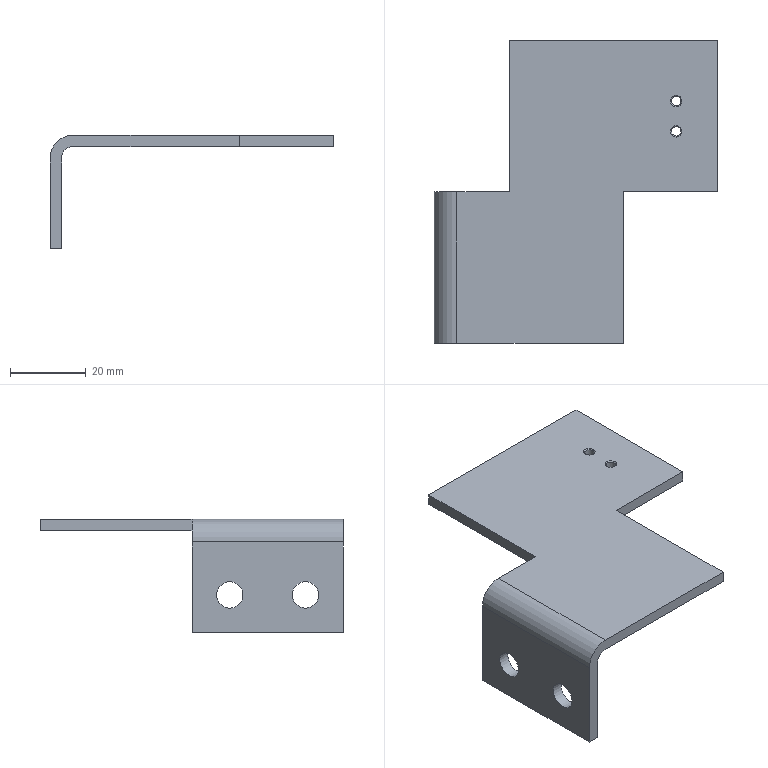Part | NX | features 5003_220_Bracket 2 | 1 solid | 20 faces | box 75 x 80 x 30 mm | volume 15347 mm3 | plane 12 | cylinder 6 | cone 2 | commonest cylinder face diameters 2.5 x2 7 x2 6 x1 12 x1
STEP:
#1=CARTESIAN_POINT('',(268.825,-58.6,-25.));
#2=VERTEX_POINT('',#1);
#3=CARTESIAN_POINT('',(268.825,-58.6,-22.));
#4=VERTEX_POINT('',#3);
#5=CARTESIAN_POINT('',(268.825,-58.6,-72.));
#6=DIRECTION('',(0.,0.,1.));
#7=VECTOR('',#6,1000.);
#8=LINE('',#5,#7);
#9=EDGE_CURVE('',#2,#4,#8,.T.);
#10=ORIENTED_EDGE('',*,*,#9,.F.);
#11=CARTESIAN_POINT('',(268.825,-18.6,-25.));
#12=VERTEX_POINT('',#11);
#13=CARTESIAN_POINT('',(268.825,-98.6,-25.));
#14=DIRECTION('',(0.,1.,0.));
#15=VECTOR('',#14,1000.);
#16=LINE('',#13,#15);
#17=EDGE_CURVE('',#2,#12,#16,.T.);
#18=ORIENTED_EDGE('',*,*,#17,.T.);
#19=CARTESIAN_POINT('',(268.825,-18.6,-22.));
#20=VERTEX_POINT('',#19);
#21=CARTESIAN_POINT('',(268.825,-18.6,-22.));
#22=DIRECTION('',(0.,0.,1.));
#23=VECTOR('',#22,1000.);
#24=LINE('',#21,#23);
#25=EDGE_CURVE('',#12,#20,#24,.T.);
#26=ORIENTED_EDGE('',*,*,#25,.T.);
#27=CARTESIAN_POINT('',(268.825,-98.6,-22.));
#28=DIRECTION('',(0.,1.,0.));
#29=VECTOR('',#28,1000.);
#30=LINE('',#27,#29);
#31=EDGE_CURVE('',#4,#20,#30,.T.);
#32=ORIENTED_EDGE('',*,*,#31,.F.);
#33=EDGE_LOOP('',(#10,#18,#26,#32));
#34=FACE_BOUND('',#33,.T.);
#35=CARTESIAN_POINT('',(268.825,-98.6,-22.));
#36=DIRECTION('',(-1.,0.,0.));
#37=DIRECTION('',(0.,-1.,0.));
#38=AXIS2_PLACEMENT_3D('',#35,#36,#37);
#39=PLANE('',#38);
#40=ADVANCED_FACE('',(#34),#39,.F.);
#41=CARTESIAN_POINT('',(257.825,-44.125,-22.));
#42=VERTEX_POINT('',#41);
#43=CARTESIAN_POINT('',(257.825,-42.6,-22.));
#44=DIRECTION('',(0.,0.,1.));
#45=DIRECTION('',(0.,-1.,0.));
#46=AXIS2_PLACEMENT_3D('',#43,#44,#45);
#47=CIRCLE('',#46,1.525);
#48=EDGE_CURVE('',#42,#42,#47,.T.);
#49=ORIENTED_EDGE('',*,*,#48,.F.);
#50=EDGE_LOOP('',(#49));
#51=FACE_BOUND('',#50,.T.);
#52=CARTESIAN_POINT('',(257.825,-36.125,-22.));
#53=VERTEX_POINT('',#52);
#54=CARTESIAN_POINT('',(257.825,-34.6,-22.));
#55=DIRECTION('',(0.,0.,1.));
#56=DIRECTION('',(0.,-1.,0.));
#57=AXIS2_PLACEMENT_3D('',#54,#55,#56);
#58=CIRCLE('',#57,1.525);
#59=EDGE_CURVE('',#53,#53,#58,.T.);
#60=ORIENTED_EDGE('',*,*,#59,.F.);
#61=EDGE_LOOP('',(#60));
#62=FACE_BOUND('',#61,.T.);
#63=CARTESIAN_POINT('',(243.825,-58.6,-22.));
#64=VERTEX_POINT('',#63);
#65=CARTESIAN_POINT('',(193.825,-58.6,-22.));
#66=DIRECTION('',(1.,0.,0.));
#67=VECTOR('',#66,1000.);
#68=LINE('',#65,#67);
#69=EDGE_CURVE('',#64,#4,#68,.T.);
#70=ORIENTED_EDGE('',*,*,#69,.T.);
#71=ORIENTED_EDGE('',*,*,#31,.T.);
#72=CARTESIAN_POINT('',(213.825,-18.6,-22.));
#73=VERTEX_POINT('',#72);
#74=CARTESIAN_POINT('',(199.825,-18.6,-22.));
#75=DIRECTION('',(-1.,0.,0.));
#76=VECTOR('',#75,1000.);
#77=LINE('',#74,#76);
#78=EDGE_CURVE('',#20,#73,#77,.T.);
#79=ORIENTED_EDGE('',*,*,#78,.T.);
#80=CARTESIAN_POINT('',(213.825,-58.6,-22.));
#81=VERTEX_POINT('',#80);
#82=CARTESIAN_POINT('',(213.825,-18.6,-22.));
#83=DIRECTION('',(0.,-1.,0.));
#84=VECTOR('',#83,1000.);
#85=LINE('',#82,#84);
#86=EDGE_CURVE('',#73,#81,#85,.T.);
#87=ORIENTED_EDGE('',*,*,#86,.T.);
#88=CARTESIAN_POINT('',(199.825,-58.6,-22.));
#89=VERTEX_POINT('',#88);
#90=CARTESIAN_POINT('',(173.825,-58.6,-22.));
#91=DIRECTION('',(1.,0.,0.));
#92=VECTOR('',#91,1000.);
#93=LINE('',#90,#92);
#94=EDGE_CURVE('',#89,#81,#93,.T.);
#95=ORIENTED_EDGE('',*,*,#94,.F.);
#96=CARTESIAN_POINT('',(199.825,-98.6,-22.));
#97=VERTEX_POINT('',#96);
#98=CARTESIAN_POINT('',(199.825,-98.6,-22.));
#99=DIRECTION('',(0.,1.,0.));
#100=VECTOR('',#99,1000.);
#101=LINE('',#98,#100);
#102=EDGE_CURVE('',#97,#89,#101,.T.);
#103=ORIENTED_EDGE('',*,*,#102,.F.);
#104=CARTESIAN_POINT('',(243.825,-98.6,-22.));
#105=VERTEX_POINT('',#104);
#106=CARTESIAN_POINT('',(199.825,-98.6,-22.));
#107=DIRECTION('',(-1.,0.,0.));
#108=VECTOR('',#107,1000.);
#109=LINE('',#106,#108);
#110=EDGE_CURVE('',#105,#97,#109,.T.);
#111=ORIENTED_EDGE('',*,*,#110,.F.);
#112=CARTESIAN_POINT('',(243.825,-18.6,-22.));
#113=DIRECTION('',(0.,-1.,0.));
#114=VECTOR('',#113,1000.);
#115=LINE('',#112,#114);
#116=EDGE_CURVE('',#64,#105,#115,.T.);
#117=ORIENTED_EDGE('',*,*,#116,.F.);
#118=EDGE_LOOP('',(#70,#71,#79,#87,#95,#103,#111,#117));
#119=FACE_BOUND('',#118,.T.);
#120=CARTESIAN_POINT('',(199.825,-98.6,-22.));
#121=DIRECTION('',(0.,0.,-1.));
#122=DIRECTION('',(0.,1.,0.));
#123=AXIS2_PLACEMENT_3D('',#120,#121,#122);
#124=PLANE('',#123);
#125=ADVANCED_FACE('',(#51,#62,#119),#124,.F.);
#126=CARTESIAN_POINT('',(257.825,-43.85,-25.));
#127=VERTEX_POINT('',#126);
#128=CARTESIAN_POINT('',(257.825,-42.6,-25.));
#129=DIRECTION('',(0.,0.,1.));
#130=DIRECTION('',(0.,-1.,0.));
#131=AXIS2_PLACEMENT_3D('',#128,#129,#130);
#132=CIRCLE('',#131,1.25);
#133=EDGE_CURVE('',#127,#127,#132,.T.);
#134=ORIENTED_EDGE('',*,*,#133,.T.);
#135=EDGE_LOOP('',(#134));
#136=FACE_BOUND('',#135,.T.);
#137=CARTESIAN_POINT('',(257.825,-35.85,-25.));
#138=VERTEX_POINT('',#137);
#139=CARTESIAN_POINT('',(257.825,-34.6,-25.));
#140=DIRECTION('',(0.,0.,1.));
#141=DIRECTION('',(0.,-1.,0.));
#142=AXIS2_PLACEMENT_3D('',#139,#140,#141);
#143=CIRCLE('',#142,1.25);
#144=EDGE_CURVE('',#138,#138,#143,.T.);
#145=ORIENTED_EDGE('',*,*,#144,.T.);
#146=EDGE_LOOP('',(#145));
#147=FACE_BOUND('',#146,.T.);
#148=CARTESIAN_POINT('',(243.825,-58.6,-25.));
#149=VERTEX_POINT('',#148);
#150=CARTESIAN_POINT('',(199.825,-58.6,-25.));
#151=DIRECTION('',(1.,0.,0.));
#152=VECTOR('',#151,1000.);
#153=LINE('',#150,#152);
#154=EDGE_CURVE('',#149,#2,#153,.T.);
#155=ORIENTED_EDGE('',*,*,#154,.F.);
#156=CARTESIAN_POINT('',(243.825,-98.6,-25.));
#157=VERTEX_POINT('',#156);
#158=CARTESIAN_POINT('',(243.825,-98.6,-25.));
#159=DIRECTION('',(0.,-1.,0.));
#160=VECTOR('',#159,1000.);
#161=LINE('',#158,#160);
#162=EDGE_CURVE('',#149,#157,#161,.T.);
#163=ORIENTED_EDGE('',*,*,#162,.T.);
#164=CARTESIAN_POINT('',(199.825,-98.6,-25.));
#165=VERTEX_POINT('',#164);
#166=CARTESIAN_POINT('',(199.825,-98.6,-25.));
#167=DIRECTION('',(1.,0.,0.));
#168=VECTOR('',#167,1000.);
#169=LINE('',#166,#168);
#170=EDGE_CURVE('',#165,#157,#169,.T.);
#171=ORIENTED_EDGE('',*,*,#170,.F.);
#172=CARTESIAN_POINT('',(199.825,-58.6,-25.));
#173=VERTEX_POINT('',#172);
#174=CARTESIAN_POINT('',(199.825,-98.6,-25.));
#175=DIRECTION('',(0.,1.,0.));
#176=VECTOR('',#175,1000.);
#177=LINE('',#174,#176);
#178=EDGE_CURVE('',#165,#173,#177,.T.);
#179=ORIENTED_EDGE('',*,*,#178,.T.);
#180=CARTESIAN_POINT('',(213.825,-58.6,-25.));
#181=VERTEX_POINT('',#180);
#182=CARTESIAN_POINT('',(199.825,-58.6,-25.));
#183=DIRECTION('',(1.,0.,0.));
#184=VECTOR('',#183,1000.);
#185=LINE('',#182,#184);
#186=EDGE_CURVE('',#173,#181,#185,.T.);
#187=ORIENTED_EDGE('',*,*,#186,.T.);
#188=CARTESIAN_POINT('',(213.825,-18.6,-25.));
#189=VERTEX_POINT('',#188);
#190=CARTESIAN_POINT('',(213.825,-98.6,-25.));
#191=DIRECTION('',(0.,-1.,0.));
#192=VECTOR('',#191,1000.);
#193=LINE('',#190,#192);
#194=EDGE_CURVE('',#189,#181,#193,.T.);
#195=ORIENTED_EDGE('',*,*,#194,.F.);
#196=CARTESIAN_POINT('',(199.825,-18.6,-25.));
#197=DIRECTION('',(1.,0.,0.));
#198=VECTOR('',#197,1000.);
#199=LINE('',#196,#198);
#200=EDGE_CURVE('',#189,#12,#199,.T.);
#201=ORIENTED_EDGE('',*,*,#200,.T.);
#202=ORIENTED_EDGE('',*,*,#17,.F.);
#203=EDGE_LOOP('',(#155,#163,#171,#179,#187,#195,#201,#202));
#204=FACE_BOUND('',#203,.T.);
#205=CARTESIAN_POINT('',(199.825,-98.6,-25.));
#206=DIRECTION('',(0.,0.,1.));
#207=DIRECTION('',(0.,-1.,0.));
#208=AXIS2_PLACEMENT_3D('',#205,#206,#207);
#209=PLANE('',#208);
#210=ADVANCED_FACE('',(#136,#147,#204),#209,.F.);
#211=ORIENTED_EDGE('',*,*,#200,.F.);
#212=CARTESIAN_POINT('',(213.825,-18.6,-28.));
#213=DIRECTION('',(0.,0.,1.));
#214=VECTOR('',#213,1000.);
#215=LINE('',#212,#214);
#216=EDGE_CURVE('',#189,#73,#215,.T.);
#217=ORIENTED_EDGE('',*,*,#216,.T.);
#218=ORIENTED_EDGE('',*,*,#78,.F.);
#219=ORIENTED_EDGE('',*,*,#25,.F.);
#220=EDGE_LOOP('',(#211,#217,#218,#219));
#221=FACE_BOUND('',#220,.T.);
#222=CARTESIAN_POINT('',(199.825,-18.6,-28.));
#223=DIRECTION('',(0.,1.,0.));
#224=DIRECTION('',(-1.,0.,0.));
#225=AXIS2_PLACEMENT_3D('',#222,#223,#224);
#226=PLANE('',#225);
#227=ADVANCED_FACE('',(#221),#226,.T.);
#228=ORIENTED_EDGE('',*,*,#102,.T.);
#229=CARTESIAN_POINT('',(193.825,-58.6,-28.));
#230=VERTEX_POINT('',#229);
#231=CARTESIAN_POINT('',(199.825,-58.6,-28.));
#232=DIRECTION('',(0.,-1.,0.));
#233=DIRECTION('',(1.,0.,0.));
#234=AXIS2_PLACEMENT_3D('',#231,#232,#233);
#235=CIRCLE('',#234,6.);
#236=EDGE_CURVE('',#89,#230,#235,.T.);
#237=ORIENTED_EDGE('',*,*,#236,.T.);
#238=CARTESIAN_POINT('',(193.825,-98.6,-28.));
#239=VERTEX_POINT('',#238);
#240=CARTESIAN_POINT('',(193.825,-98.6,-28.));
#241=DIRECTION('',(0.,1.,0.));
#242=VECTOR('',#241,1000.);
#243=LINE('',#240,#242);
#244=EDGE_CURVE('',#239,#230,#243,.T.);
#245=ORIENTED_EDGE('',*,*,#244,.F.);
#246=CARTESIAN_POINT('',(199.825,-98.6,-28.));
#247=DIRECTION('',(0.,-1.,0.));
#248=DIRECTION('',(-1.,0.,0.));
#249=AXIS2_PLACEMENT_3D('',#246,#247,#248);
#250=CIRCLE('',#249,6.);
#251=EDGE_CURVE('',#97,#239,#250,.T.);
#252=ORIENTED_EDGE('',*,*,#251,.F.);
#253=EDGE_LOOP('',(#228,#237,#245,#252));
#254=FACE_BOUND('',#253,.T.);
#255=CARTESIAN_POINT('',(199.825,-98.6,-28.));
#256=DIRECTION('',(0.,1.,0.));
#257=DIRECTION('',(-1.,0.,0.));
#258=AXIS2_PLACEMENT_3D('',#255,#256,#257);
#259=CYLINDRICAL_SURFACE('',#258,6.);
#260=ADVANCED_FACE('',(#254),#259,.T.);
#261=CARTESIAN_POINT('',(193.825,-88.6,-38.5));
#262=VERTEX_POINT('',#261);
#263=CARTESIAN_POINT('',(193.825,-88.6,-42.));
#264=DIRECTION('',(1.,0.,0.));
#265=DIRECTION('',(0.,0.,1.));
#266=AXIS2_PLACEMENT_3D('',#263,#264,#265);
#267=CIRCLE('',#266,3.5);
#268=EDGE_CURVE('',#262,#262,#267,.T.);
#269=ORIENTED_EDGE('',*,*,#268,.T.);
#270=EDGE_LOOP('',(#269));
#271=FACE_BOUND('',#270,.T.);
#272=CARTESIAN_POINT('',(193.825,-68.6,-38.5));
#273=VERTEX_POINT('',#272);
#274=CARTESIAN_POINT('',(193.825,-68.6,-42.));
#275=DIRECTION('',(1.,0.,0.));
#276=DIRECTION('',(0.,0.,1.));
#277=AXIS2_PLACEMENT_3D('',#274,#275,#276);
#278=CIRCLE('',#277,3.5);
#279=EDGE_CURVE('',#273,#273,#278,.T.);
#280=ORIENTED_EDGE('',*,*,#279,.T.);
#281=EDGE_LOOP('',(#280));
#282=FACE_BOUND('',#281,.T.);
#283=ORIENTED_EDGE('',*,*,#244,.T.);
#284=CARTESIAN_POINT('',(193.825,-58.6,-52.));
#285=VERTEX_POINT('',#284);
#286=CARTESIAN_POINT('',(193.825,-58.6,-28.));
#287=DIRECTION('',(0.,0.,-1.));
#288=VECTOR('',#287,1000.);
#289=LINE('',#286,#288);
#290=EDGE_CURVE('',#230,#285,#289,.T.);
#291=ORIENTED_EDGE('',*,*,#290,.T.);
#292=CARTESIAN_POINT('',(193.825,-98.6,-52.));
#293=VERTEX_POINT('',#292);
#294=CARTESIAN_POINT('',(193.825,-98.6,-52.));
#295=DIRECTION('',(0.,1.,0.));
#296=VECTOR('',#295,1000.);
#297=LINE('',#294,#296);
#298=EDGE_CURVE('',#293,#285,#297,.T.);
#299=ORIENTED_EDGE('',*,*,#298,.F.);
#300=CARTESIAN_POINT('',(193.825,-98.6,-28.));
#301=DIRECTION('',(0.,0.,-1.));
#302=VECTOR('',#301,1000.);
#303=LINE('',#300,#302);
#304=EDGE_CURVE('',#239,#293,#303,.T.);
#305=ORIENTED_EDGE('',*,*,#304,.F.);
#306=EDGE_LOOP('',(#283,#291,#299,#305));
#307=FACE_BOUND('',#306,.T.);
#308=CARTESIAN_POINT('',(193.825,-98.6,-28.));
#309=DIRECTION('',(1.,0.,0.));
#310=DIRECTION('',(0.,0.,1.));
#311=AXIS2_PLACEMENT_3D('',#308,#309,#310);
#312=PLANE('',#311);
#313=ADVANCED_FACE('',(#271,#282,#307),#312,.F.);
#314=ORIENTED_EDGE('',*,*,#298,.T.);
#315=CARTESIAN_POINT('',(196.825,-58.6,-52.));
#316=VERTEX_POINT('',#315);
#317=CARTESIAN_POINT('',(193.825,-58.6,-52.));
#318=DIRECTION('',(1.,0.,0.));
#319=VECTOR('',#318,1000.);
#320=LINE('',#317,#319);
#321=EDGE_CURVE('',#285,#316,#320,.T.);
#322=ORIENTED_EDGE('',*,*,#321,.T.);
#323=CARTESIAN_POINT('',(196.825,-98.6,-52.));
#324=VERTEX_POINT('',#323);
#325=CARTESIAN_POINT('',(196.825,-98.6,-52.));
#326=DIRECTION('',(0.,1.,0.));
#327=VECTOR('',#326,1000.);
#328=LINE('',#325,#327);
#329=EDGE_CURVE('',#324,#316,#328,.T.);
#330=ORIENTED_EDGE('',*,*,#329,.F.);
#331=CARTESIAN_POINT('',(193.825,-98.6,-52.));
#332=DIRECTION('',(1.,0.,0.));
#333=VECTOR('',#332,1000.);
#334=LINE('',#331,#333);
#335=EDGE_CURVE('',#293,#324,#334,.T.);
#336=ORIENTED_EDGE('',*,*,#335,.F.);
#337=EDGE_LOOP('',(#314,#322,#330,#336));
#338=FACE_BOUND('',#337,.T.);
#339=CARTESIAN_POINT('',(193.825,-98.6,-52.));
#340=DIRECTION('',(0.,0.,1.));
#341=DIRECTION('',(0.,-1.,0.));
#342=AXIS2_PLACEMENT_3D('',#339,#340,#341);
#343=PLANE('',#342);
#344=ADVANCED_FACE('',(#338),#343,.F.);
#345=CARTESIAN_POINT('',(196.825,-88.6,-38.5));
#346=VERTEX_POINT('',#345);
#347=CARTESIAN_POINT('',(196.825,-88.6,-42.));
#348=DIRECTION('',(1.,0.,0.));
#349=DIRECTION('',(0.,0.,1.));
#350=AXIS2_PLACEMENT_3D('',#347,#348,#349);
#351=CIRCLE('',#350,3.5);
#352=EDGE_CURVE('',#346,#346,#351,.T.);
#353=ORIENTED_EDGE('',*,*,#352,.F.);
#354=EDGE_LOOP('',(#353));
#355=FACE_BOUND('',#354,.T.);
#356=CARTESIAN_POINT('',(196.825,-68.6,-38.5));
#357=VERTEX_POINT('',#356);
#358=CARTESIAN_POINT('',(196.825,-68.6,-42.));
#359=DIRECTION('',(1.,0.,0.));
#360=DIRECTION('',(0.,0.,1.));
#361=AXIS2_PLACEMENT_3D('',#358,#359,#360);
#362=CIRCLE('',#361,3.5);
#363=EDGE_CURVE('',#357,#357,#362,.T.);
#364=ORIENTED_EDGE('',*,*,#363,.F.);
#365=EDGE_LOOP('',(#364));
#366=FACE_BOUND('',#365,.T.);
#367=ORIENTED_EDGE('',*,*,#329,.T.);
#368=CARTESIAN_POINT('',(196.825,-58.6,-28.));
#369=VERTEX_POINT('',#368);
#370=CARTESIAN_POINT('',(196.825,-58.6,-52.));
#371=DIRECTION('',(0.,0.,1.));
#372=VECTOR('',#371,1000.);
#373=LINE('',#370,#372);
#374=EDGE_CURVE('',#316,#369,#373,.T.);
#375=ORIENTED_EDGE('',*,*,#374,.T.);
#376=CARTESIAN_POINT('',(196.825,-98.6,-28.));
#377=VERTEX_POINT('',#376);
#378=CARTESIAN_POINT('',(196.825,-98.6,-28.));
#379=DIRECTION('',(0.,1.,0.));
#380=VECTOR('',#379,1000.);
#381=LINE('',#378,#380);
#382=EDGE_CURVE('',#377,#369,#381,.T.);
#383=ORIENTED_EDGE('',*,*,#382,.F.);
#384=CARTESIAN_POINT('',(196.825,-98.6,-52.));
#385=DIRECTION('',(0.,0.,1.));
#386=VECTOR('',#385,1000.);
#387=LINE('',#384,#386);
#388=EDGE_CURVE('',#324,#377,#387,.T.);
#389=ORIENTED_EDGE('',*,*,#388,.F.);
#390=EDGE_LOOP('',(#367,#375,#383,#389));
#391=FACE_BOUND('',#390,.T.);
#392=CARTESIAN_POINT('',(196.825,-98.6,-52.));
#393=DIRECTION('',(-1.,0.,0.));
#394=DIRECTION('',(0.,0.,-1.));
#395=AXIS2_PLACEMENT_3D('',#392,#393,#394);
#396=PLANE('',#395);
#397=ADVANCED_FACE('',(#355,#366,#391),#396,.F.);
#398=ORIENTED_EDGE('',*,*,#382,.T.);
#399=CARTESIAN_POINT('',(199.825,-58.6,-28.));
#400=DIRECTION('',(0.,-1.,0.));
#401=DIRECTION('',(1.,0.,0.));
#402=AXIS2_PLACEMENT_3D('',#399,#400,#401);
#403=CIRCLE('',#402,3.);
#404=EDGE_CURVE('',#369,#173,#403,.F.);
#405=ORIENTED_EDGE('',*,*,#404,.T.);
#406=ORIENTED_EDGE('',*,*,#178,.F.);
#407=CARTESIAN_POINT('',(199.825,-98.6,-28.));
#408=DIRECTION('',(0.,1.,0.));
#409=DIRECTION('',(-1.,0.,0.));
#410=AXIS2_PLACEMENT_3D('',#407,#408,#409);
#411=CIRCLE('',#410,3.);
#412=EDGE_CURVE('',#377,#165,#411,.T.);
#413=ORIENTED_EDGE('',*,*,#412,.F.);
#414=EDGE_LOOP('',(#398,#405,#406,#413));
#415=FACE_BOUND('',#414,.T.);
#416=CARTESIAN_POINT('',(199.825,-98.6,-28.));
#417=DIRECTION('',(0.,1.,0.));
#418=DIRECTION('',(-1.,0.,0.));
#419=AXIS2_PLACEMENT_3D('',#416,#417,#418);
#420=CYLINDRICAL_SURFACE('',#419,3.);
#421=ADVANCED_FACE('',(#415),#420,.F.);
#422=ORIENTED_EDGE('',*,*,#170,.T.);
#423=CARTESIAN_POINT('',(243.825,-98.6,-28.));
#424=DIRECTION('',(0.,0.,1.));
#425=VECTOR('',#424,1000.);
#426=LINE('',#423,#425);
#427=EDGE_CURVE('',#157,#105,#426,.T.);
#428=ORIENTED_EDGE('',*,*,#427,.T.);
#429=ORIENTED_EDGE('',*,*,#110,.T.);
#430=ORIENTED_EDGE('',*,*,#251,.T.);
#431=ORIENTED_EDGE('',*,*,#304,.T.);
#432=ORIENTED_EDGE('',*,*,#335,.T.);
#433=ORIENTED_EDGE('',*,*,#388,.T.);
#434=ORIENTED_EDGE('',*,*,#412,.T.);
#435=EDGE_LOOP('',(#422,#428,#429,#430,#431,#432,#433,#434));
#436=FACE_BOUND('',#435,.T.);
#437=CARTESIAN_POINT('',(199.825,-98.6,-28.));
#438=DIRECTION('',(0.,1.,0.));
#439=DIRECTION('',(-1.,0.,0.));
#440=AXIS2_PLACEMENT_3D('',#437,#438,#439);
#441=PLANE('',#440);
#442=ADVANCED_FACE('',(#436),#441,.F.);
#443=ORIENTED_EDGE('',*,*,#279,.F.);
#444=EDGE_LOOP('',(#443));
#445=FACE_BOUND('',#444,.T.);
#446=ORIENTED_EDGE('',*,*,#363,.T.);
#447=EDGE_LOOP('',(#446));
#448=FACE_BOUND('',#447,.T.);
#449=CARTESIAN_POINT('',(193.825,-68.6,-42.));
#450=DIRECTION('',(1.,0.,0.));
#451=DIRECTION('',(0.,0.,1.));
#452=AXIS2_PLACEMENT_3D('',#449,#450,#451);
#453=CYLINDRICAL_SURFACE('',#452,3.5);
#454=ADVANCED_FACE('',(#445,#448),#453,.F.);
#455=ORIENTED_EDGE('',*,*,#268,.F.);
#456=EDGE_LOOP('',(#455));
#457=FACE_BOUND('',#456,.T.);
#458=ORIENTED_EDGE('',*,*,#352,.T.);
#459=EDGE_LOOP('',(#458));
#460=FACE_BOUND('',#459,.T.);
#461=CARTESIAN_POINT('',(193.825,-88.6,-42.));
#462=DIRECTION('',(1.,0.,0.));
#463=DIRECTION('',(0.,0.,1.));
#464=AXIS2_PLACEMENT_3D('',#461,#462,#463);
#465=CYLINDRICAL_SURFACE('',#464,3.5);
#466=ADVANCED_FACE('',(#457,#460),#465,.F.);
#467=CARTESIAN_POINT('',(257.825,-35.85,-22.275));
#468=VERTEX_POINT('',#467);
#469=CARTESIAN_POINT('',(257.825,-34.6,-22.275));
#470=DIRECTION('',(0.,0.,1.));
#471=DIRECTION('',(0.,-1.,0.));
#472=AXIS2_PLACEMENT_3D('',#469,#470,#471);
#473=CIRCLE('',#472,1.25);
#474=EDGE_CURVE('',#468,#468,#473,.T.);
#475=ORIENTED_EDGE('',*,*,#474,.T.);
#476=EDGE_LOOP('',(#475));
#477=FACE_BOUND('',#476,.T.);
#478=ORIENTED_EDGE('',*,*,#144,.F.);
#479=EDGE_LOOP('',(#478));
#480=FACE_BOUND('',#479,.T.);
#481=CARTESIAN_POINT('',(257.825,-34.6,-22.));
#482=DIRECTION('',(0.,0.,1.));
#483=DIRECTION('',(0.,-1.,0.));
#484=AXIS2_PLACEMENT_3D('',#481,#482,#483);
#485=CYLINDRICAL_SURFACE('',#484,1.25);
#486=ADVANCED_FACE('',(#477,#480),#485,.F.);
#487=ORIENTED_EDGE('',*,*,#474,.F.);
#488=EDGE_LOOP('',(#487));
#489=FACE_BOUND('',#488,.T.);
#490=ORIENTED_EDGE('',*,*,#59,.T.);
#491=EDGE_LOOP('',(#490));
#492=FACE_BOUND('',#491,.T.);
#493=CARTESIAN_POINT('',(257.825,-34.6,-22.));
#494=DIRECTION('',(0.,0.,1.));
#495=DIRECTION('',(0.,-1.,0.));
#496=AXIS2_PLACEMENT_3D('',#493,#494,#495);
#497=CONICAL_SURFACE('',#496,1.525,0.7854);
#498=ADVANCED_FACE('',(#489,#492),#497,.F.);
#499=CARTESIAN_POINT('',(257.825,-43.85,-22.275));
#500=VERTEX_POINT('',#499);
#501=CARTESIAN_POINT('',(257.825,-42.6,-22.275));
#502=DIRECTION('',(0.,0.,1.));
#503=DIRECTION('',(0.,-1.,0.));
#504=AXIS2_PLACEMENT_3D('',#501,#502,#503);
#505=CIRCLE('',#504,1.25);
#506=EDGE_CURVE('',#500,#500,#505,.T.);
#507=ORIENTED_EDGE('',*,*,#506,.T.);
#508=EDGE_LOOP('',(#507));
#509=FACE_BOUND('',#508,.T.);
#510=ORIENTED_EDGE('',*,*,#133,.F.);
#511=EDGE_LOOP('',(#510));
#512=FACE_BOUND('',#511,.T.);
#513=CARTESIAN_POINT('',(257.825,-42.6,-22.));
#514=DIRECTION('',(0.,0.,1.));
#515=DIRECTION('',(0.,-1.,0.));
#516=AXIS2_PLACEMENT_3D('',#513,#514,#515);
#517=CYLINDRICAL_SURFACE('',#516,1.25);
#518=ADVANCED_FACE('',(#509,#512),#517,.F.);
#519=ORIENTED_EDGE('',*,*,#506,.F.);
#520=EDGE_LOOP('',(#519));
#521=FACE_BOUND('',#520,.T.);
#522=ORIENTED_EDGE('',*,*,#48,.T.);
#523=EDGE_LOOP('',(#522));
#524=FACE_BOUND('',#523,.T.);
#525=CARTESIAN_POINT('',(257.825,-42.6,-22.));
#526=DIRECTION('',(0.,0.,1.));
#527=DIRECTION('',(0.,-1.,0.));
#528=AXIS2_PLACEMENT_3D('',#525,#526,#527);
#529=CONICAL_SURFACE('',#528,1.525,0.7854);
#530=ADVANCED_FACE('',(#521,#524),#529,.F.);
#531=ORIENTED_EDGE('',*,*,#94,.T.);
#532=CARTESIAN_POINT('',(213.825,-58.6,-72.));
#533=DIRECTION('',(0.,0.,1.));
#534=VECTOR('',#533,1000.);
#535=LINE('',#532,#534);
#536=EDGE_CURVE('',#181,#81,#535,.T.);
#537=ORIENTED_EDGE('',*,*,#536,.F.);
#538=ORIENTED_EDGE('',*,*,#186,.F.);
#539=ORIENTED_EDGE('',*,*,#404,.F.);
#540=ORIENTED_EDGE('',*,*,#374,.F.);
#541=ORIENTED_EDGE('',*,*,#321,.F.);
#542=ORIENTED_EDGE('',*,*,#290,.F.);
#543=ORIENTED_EDGE('',*,*,#236,.F.);
#544=EDGE_LOOP('',(#531,#537,#538,#539,#540,#541,#542,#543));
#545=FACE_BOUND('',#544,.T.);
#546=CARTESIAN_POINT('',(173.825,-58.6,-72.));
#547=DIRECTION('',(0.,-1.,0.));
#548=DIRECTION('',(1.,0.,0.));
#549=AXIS2_PLACEMENT_3D('',#546,#547,#548);
#550=PLANE('',#549);
#551=ADVANCED_FACE('',(#545),#550,.F.);
#552=ORIENTED_EDGE('',*,*,#194,.T.);
#553=ORIENTED_EDGE('',*,*,#536,.T.);
#554=ORIENTED_EDGE('',*,*,#86,.F.);
#555=ORIENTED_EDGE('',*,*,#216,.F.);
#556=EDGE_LOOP('',(#552,#553,#554,#555));
#557=FACE_BOUND('',#556,.T.);
#558=CARTESIAN_POINT('',(213.825,-18.6,-72.));
#559=DIRECTION('',(-1.,0.,0.));
#560=DIRECTION('',(0.,-1.,0.));
#561=AXIS2_PLACEMENT_3D('',#558,#559,#560);
#562=PLANE('',#561);
#563=ADVANCED_FACE('',(#557),#562,.T.);
#564=ORIENTED_EDGE('',*,*,#154,.T.);
#565=ORIENTED_EDGE('',*,*,#9,.T.);
#566=ORIENTED_EDGE('',*,*,#69,.F.);
#567=CARTESIAN_POINT('',(243.825,-58.6,-72.));
#568=DIRECTION('',(0.,0.,1.));
#569=VECTOR('',#568,1000.);
#570=LINE('',#567,#569);
#571=EDGE_CURVE('',#149,#64,#570,.T.);
#572=ORIENTED_EDGE('',*,*,#571,.F.);
#573=EDGE_LOOP('',(#564,#565,#566,#572));
#574=FACE_BOUND('',#573,.T.);
#575=CARTESIAN_POINT('',(193.825,-58.6,-72.));
#576=DIRECTION('',(0.,-1.,0.));
#577=DIRECTION('',(1.,0.,0.));
#578=AXIS2_PLACEMENT_3D('',#575,#576,#577);
#579=PLANE('',#578);
#580=ADVANCED_FACE('',(#574),#579,.T.);
#581=ORIENTED_EDGE('',*,*,#571,.T.);
#582=ORIENTED_EDGE('',*,*,#116,.T.);
#583=ORIENTED_EDGE('',*,*,#427,.F.);
#584=ORIENTED_EDGE('',*,*,#162,.F.);
#585=EDGE_LOOP('',(#581,#582,#583,#584));
#586=FACE_BOUND('',#585,.T.);
#587=CARTESIAN_POINT('',(243.825,-18.6,-72.));
#588=DIRECTION('',(-1.,0.,0.));
#589=DIRECTION('',(0.,-1.,0.));
#590=AXIS2_PLACEMENT_3D('',#587,#588,#589);
#591=PLANE('',#590);
#592=ADVANCED_FACE('',(#586),#591,.F.);
#593=CLOSED_SHELL('',(#40,#125,#210,#227,#260,#313,#344,#397,#421,#442,#454,#466,#486,#498,#518,#530,#551,#563,#580,#592));
#594=MANIFOLD_SOLID_BREP('',#593);
#595=(LENGTH_UNIT()NAMED_UNIT(*)SI_UNIT(.MILLI.,.METRE.));
#596=UNCERTAINTY_MEASURE_WITH_UNIT(LENGTH_MEASURE(0.00001),#595,'','');
#597=(NAMED_UNIT(*)PLANE_ANGLE_UNIT()SI_UNIT($,.RADIAN.));
#598=(NAMED_UNIT(*)SI_UNIT($,.STERADIAN.)SOLID_ANGLE_UNIT());
#599=(GEOMETRIC_REPRESENTATION_CONTEXT(3)GLOBAL_UNCERTAINTY_ASSIGNED_CONTEXT((#596))GLOBAL_UNIT_ASSIGNED_CONTEXT((#595,#597,#598))REPRESENTATION_CONTEXT('',''));
#600=ADVANCED_BREP_SHAPE_REPRESENTATION('',(#594),#599);